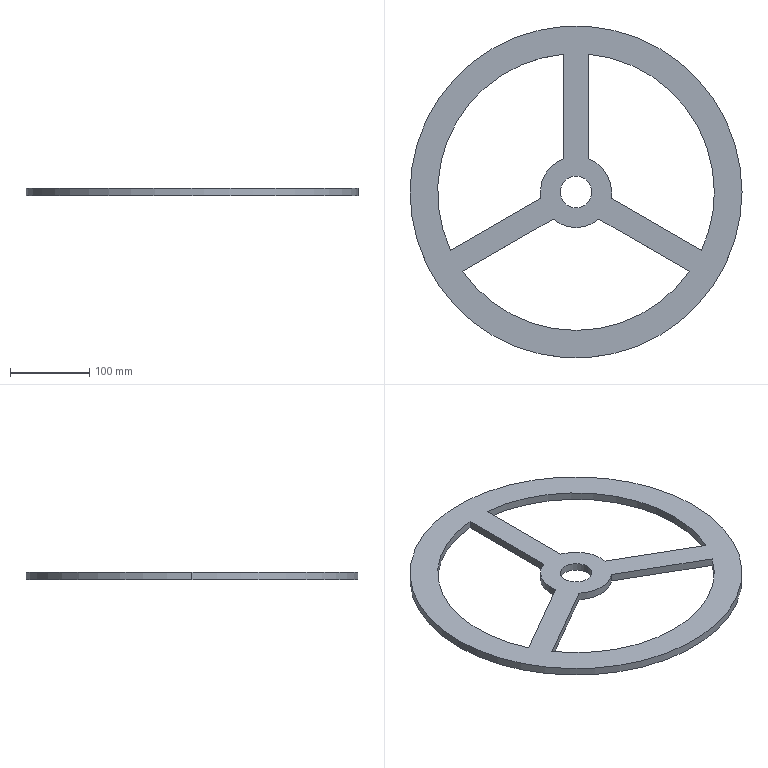Part | SolidWorks | features BaseBody 1 | 1 solid | 20 faces | box 420 x 420 x 10 mm | volume 593937 mm3 | cylinder 12 | plane 8 | commonest cylinder face diameters 90 x4 350 x4 40 x2 420 x2
STEP:
#1=CARTESIAN_POINT('',(20.,0.,0.));
#2=VERTEX_POINT('',#1);
#3=CARTESIAN_POINT('',(-20.,0.,0.));
#4=VERTEX_POINT('',#3);
#5=CARTESIAN_POINT('',(0.,0.,0.));
#6=DIRECTION('',(0.,0.,-1.));
#7=DIRECTION('',(1.,0.,0.));
#8=AXIS2_PLACEMENT_3D('',#5,#6,#7);
#9=CIRCLE('',#8,20.);
#10=EDGE_CURVE('',#2,#4,#9,.T.);
#11=ORIENTED_EDGE('',*,*,#10,.T.);
#12=CARTESIAN_POINT('',(-20.,0.,10.));
#13=VERTEX_POINT('',#12);
#14=CARTESIAN_POINT('',(-20.,0.,0.));
#15=DIRECTION('',(0.,0.,1.));
#16=VECTOR('',#15,1000.);
#17=LINE('',#14,#16);
#18=EDGE_CURVE('',#4,#13,#17,.T.);
#19=ORIENTED_EDGE('',*,*,#18,.T.);
#20=CARTESIAN_POINT('',(20.,0.,10.));
#21=VERTEX_POINT('',#20);
#22=CARTESIAN_POINT('',(0.,0.,10.));
#23=DIRECTION('',(0.,0.,-1.));
#24=DIRECTION('',(1.,0.,0.));
#25=AXIS2_PLACEMENT_3D('',#22,#23,#24);
#26=CIRCLE('',#25,20.);
#27=EDGE_CURVE('',#21,#13,#26,.T.);
#28=ORIENTED_EDGE('',*,*,#27,.F.);
#29=CARTESIAN_POINT('',(20.,0.,0.));
#30=DIRECTION('',(0.,0.,1.));
#31=VECTOR('',#30,1000.);
#32=LINE('',#29,#31);
#33=EDGE_CURVE('',#2,#21,#32,.T.);
#34=ORIENTED_EDGE('',*,*,#33,.F.);
#35=EDGE_LOOP('',(#11,#19,#28,#34));
#36=FACE_OUTER_BOUND('',#35,.T.);
#37=CARTESIAN_POINT('',(0.,0.,0.));
#38=DIRECTION('',(0.,0.,1.));
#39=DIRECTION('',(1.,0.,0.));
#40=AXIS2_PLACEMENT_3D('',#37,#38,#39);
#41=CYLINDRICAL_SURFACE('',#40,20.);
#42=ADVANCED_FACE('',(#36),#41,.F.);
#43=CARTESIAN_POINT('',(15.251,174.334,0.));
#44=VERTEX_POINT('',#43);
#45=CARTESIAN_POINT('',(175.,0.,0.));
#46=VERTEX_POINT('',#45);
#47=CARTESIAN_POINT('',(0.,0.,0.));
#48=DIRECTION('',(0.,0.,-1.));
#49=DIRECTION('',(1.,0.,0.));
#50=AXIS2_PLACEMENT_3D('',#47,#48,#49);
#51=CIRCLE('',#50,175.);
#52=EDGE_CURVE('',#44,#46,#51,.T.);
#53=ORIENTED_EDGE('',*,*,#52,.T.);
#54=CARTESIAN_POINT('',(175.,0.,10.));
#55=VERTEX_POINT('',#54);
#56=CARTESIAN_POINT('',(175.,0.,0.));
#57=DIRECTION('',(0.,0.,1.));
#58=VECTOR('',#57,1000.);
#59=LINE('',#56,#58);
#60=EDGE_CURVE('',#46,#55,#59,.T.);
#61=ORIENTED_EDGE('',*,*,#60,.T.);
#62=CARTESIAN_POINT('',(15.251,174.334,10.));
#63=VERTEX_POINT('',#62);
#64=CARTESIAN_POINT('',(0.,0.,10.));
#65=DIRECTION('',(0.,0.,-1.));
#66=DIRECTION('',(1.,0.,0.));
#67=AXIS2_PLACEMENT_3D('',#64,#65,#66);
#68=CIRCLE('',#67,175.);
#69=EDGE_CURVE('',#63,#55,#68,.T.);
#70=ORIENTED_EDGE('',*,*,#69,.F.);
#71=CARTESIAN_POINT('',(15.251,174.334,0.));
#72=DIRECTION('',(0.,0.,1.));
#73=VECTOR('',#72,1000.);
#74=LINE('',#71,#73);
#75=EDGE_CURVE('',#44,#63,#74,.T.);
#76=ORIENTED_EDGE('',*,*,#75,.F.);
#77=EDGE_LOOP('',(#53,#61,#70,#76));
#78=FACE_OUTER_BOUND('',#77,.T.);
#79=CARTESIAN_POINT('',(0.,0.,0.));
#80=DIRECTION('',(0.,0.,1.));
#81=DIRECTION('',(1.,0.,0.));
#82=AXIS2_PLACEMENT_3D('',#79,#80,#81);
#83=CYLINDRICAL_SURFACE('',#82,175.);
#84=ADVANCED_FACE('',(#78),#83,.F.);
#85=CARTESIAN_POINT('',(44.29,-7.961,0.));
#86=VERTEX_POINT('',#85);
#87=CARTESIAN_POINT('',(45.,0.,0.));
#88=VERTEX_POINT('',#87);
#89=CARTESIAN_POINT('',(0.,0.,0.));
#90=DIRECTION('',(0.,0.,1.));
#91=DIRECTION('',(1.,0.,0.));
#92=AXIS2_PLACEMENT_3D('',#89,#90,#91);
#93=CIRCLE('',#92,45.);
#94=EDGE_CURVE('',#86,#88,#93,.T.);
#95=ORIENTED_EDGE('',*,*,#94,.T.);
#96=CARTESIAN_POINT('',(45.,0.,10.));
#97=VERTEX_POINT('',#96);
#98=CARTESIAN_POINT('',(45.,0.,0.));
#99=DIRECTION('',(0.,0.,1.));
#100=VECTOR('',#99,1000.);
#101=LINE('',#98,#100);
#102=EDGE_CURVE('',#88,#97,#101,.T.);
#103=ORIENTED_EDGE('',*,*,#102,.T.);
#104=CARTESIAN_POINT('',(44.29,-7.961,10.));
#105=VERTEX_POINT('',#104);
#106=CARTESIAN_POINT('',(0.,0.,10.));
#107=DIRECTION('',(0.,0.,-1.));
#108=DIRECTION('',(1.,0.,0.));
#109=AXIS2_PLACEMENT_3D('',#106,#107,#108);
#110=CIRCLE('',#109,45.);
#111=EDGE_CURVE('',#97,#105,#110,.T.);
#112=ORIENTED_EDGE('',*,*,#111,.T.);
#113=CARTESIAN_POINT('',(44.29,-7.961,0.));
#114=DIRECTION('',(0.,0.,-1.));
#115=VECTOR('',#114,1000.);
#116=LINE('',#113,#115);
#117=EDGE_CURVE('',#105,#86,#116,.T.);
#118=ORIENTED_EDGE('',*,*,#117,.T.);
#119=EDGE_LOOP('',(#95,#103,#112,#118));
#120=FACE_OUTER_BOUND('',#119,.T.);
#121=CARTESIAN_POINT('',(0.,0.,0.));
#122=DIRECTION('',(0.,0.,1.));
#123=DIRECTION('',(1.,0.,0.));
#124=AXIS2_PLACEMENT_3D('',#121,#122,#123);
#125=CYLINDRICAL_SURFACE('',#124,45.);
#126=ADVANCED_FACE('',(#120),#125,.T.);
#127=CARTESIAN_POINT('',(210.,0.,0.));
#128=VERTEX_POINT('',#127);
#129=CARTESIAN_POINT('',(-210.,0.,0.));
#130=VERTEX_POINT('',#129);
#131=CARTESIAN_POINT('',(0.,0.,0.));
#132=DIRECTION('',(0.,0.,1.));
#133=DIRECTION('',(1.,0.,0.));
#134=AXIS2_PLACEMENT_3D('',#131,#132,#133);
#135=CIRCLE('',#134,210.);
#136=EDGE_CURVE('',#128,#130,#135,.T.);
#137=ORIENTED_EDGE('',*,*,#136,.T.);
#138=CARTESIAN_POINT('',(-210.,0.,10.));
#139=VERTEX_POINT('',#138);
#140=CARTESIAN_POINT('',(-210.,0.,0.));
#141=DIRECTION('',(0.,0.,1.));
#142=VECTOR('',#141,1000.);
#143=LINE('',#140,#142);
#144=EDGE_CURVE('',#130,#139,#143,.T.);
#145=ORIENTED_EDGE('',*,*,#144,.T.);
#146=CARTESIAN_POINT('',(210.,0.,10.));
#147=VERTEX_POINT('',#146);
#148=CARTESIAN_POINT('',(0.,0.,10.));
#149=DIRECTION('',(0.,0.,-1.));
#150=DIRECTION('',(1.,0.,0.));
#151=AXIS2_PLACEMENT_3D('',#148,#149,#150);
#152=CIRCLE('',#151,210.);
#153=EDGE_CURVE('',#139,#147,#152,.T.);
#154=ORIENTED_EDGE('',*,*,#153,.T.);
#155=CARTESIAN_POINT('',(210.,0.,0.));
#156=DIRECTION('',(0.,0.,1.));
#157=VECTOR('',#156,1000.);
#158=LINE('',#155,#157);
#159=EDGE_CURVE('',#128,#147,#158,.T.);
#160=ORIENTED_EDGE('',*,*,#159,.F.);
#161=EDGE_LOOP('',(#137,#145,#154,#160));
#162=FACE_OUTER_BOUND('',#161,.T.);
#163=CARTESIAN_POINT('',(0.,0.,0.));
#164=DIRECTION('',(0.,0.,1.));
#165=DIRECTION('',(1.,0.,0.));
#166=AXIS2_PLACEMENT_3D('',#163,#164,#165);
#167=CYLINDRICAL_SURFACE('',#166,210.);
#168=ADVANCED_FACE('',(#162),#167,.T.);
#169=ORIENTED_EDGE('',*,*,#10,.F.);
#170=CARTESIAN_POINT('',(0.,0.,0.));
#171=DIRECTION('',(0.,0.,-1.));
#172=DIRECTION('',(1.,0.,0.));
#173=AXIS2_PLACEMENT_3D('',#170,#171,#172);
#174=CIRCLE('',#173,20.);
#175=EDGE_CURVE('',#4,#2,#174,.T.);
#176=ORIENTED_EDGE('',*,*,#175,.F.);
#177=EDGE_LOOP('',(#169,#176));
#178=FACE_BOUND('',#177,.T.);
#179=CARTESIAN_POINT('',(-15.251,42.337,0.));
#180=VERTEX_POINT('',#179);
#181=CARTESIAN_POINT('',(-44.29,-7.961,0.));
#182=VERTEX_POINT('',#181);
#183=CARTESIAN_POINT('',(0.,0.,0.));
#184=DIRECTION('',(0.,0.,1.));
#185=DIRECTION('',(1.,0.,0.));
#186=AXIS2_PLACEMENT_3D('',#183,#184,#185);
#187=CIRCLE('',#186,45.);
#188=EDGE_CURVE('',#180,#182,#187,.T.);
#189=ORIENTED_EDGE('',*,*,#188,.F.);
#190=CARTESIAN_POINT('',(-15.251,174.334,0.));
#191=VERTEX_POINT('',#190);
#192=CARTESIAN_POINT('',(-15.251,0.,0.));
#193=DIRECTION('',(0.,-1.,0.));
#194=VECTOR('',#193,1000.);
#195=LINE('',#192,#194);
#196=EDGE_CURVE('',#191,#180,#195,.T.);
#197=ORIENTED_EDGE('',*,*,#196,.F.);
#198=CARTESIAN_POINT('',(-158.603,-73.959,0.));
#199=VERTEX_POINT('',#198);
#200=CARTESIAN_POINT('',(0.,0.,0.));
#201=DIRECTION('',(0.,0.,-1.));
#202=DIRECTION('',(1.,0.,0.));
#203=AXIS2_PLACEMENT_3D('',#200,#201,#202);
#204=CIRCLE('',#203,175.);
#205=EDGE_CURVE('',#199,#191,#204,.T.);
#206=ORIENTED_EDGE('',*,*,#205,.F.);
#207=CARTESIAN_POINT('',(-44.29,-7.961,0.));
#208=DIRECTION('',(-0.866,-0.5,0.));
#209=VECTOR('',#208,1000.);
#210=LINE('',#207,#209);
#211=EDGE_CURVE('',#182,#199,#210,.T.);
#212=ORIENTED_EDGE('',*,*,#211,.F.);
#213=EDGE_LOOP('',(#189,#197,#206,#212));
#214=FACE_BOUND('',#213,.T.);
#215=CARTESIAN_POINT('',(-29.039,-34.376,0.));
#216=VERTEX_POINT('',#215);
#217=CARTESIAN_POINT('',(29.039,-34.376,0.));
#218=VERTEX_POINT('',#217);
#219=CARTESIAN_POINT('',(0.,0.,0.));
#220=DIRECTION('',(0.,0.,1.));
#221=DIRECTION('',(1.,0.,0.));
#222=AXIS2_PLACEMENT_3D('',#219,#220,#221);
#223=CIRCLE('',#222,45.);
#224=EDGE_CURVE('',#216,#218,#223,.T.);
#225=ORIENTED_EDGE('',*,*,#224,.F.);
#226=CARTESIAN_POINT('',(-143.352,-100.375,0.));
#227=VERTEX_POINT('',#226);
#228=CARTESIAN_POINT('',(-143.352,-100.375,0.));
#229=DIRECTION('',(0.866,0.5,0.));
#230=VECTOR('',#229,1000.);
#231=LINE('',#228,#230);
#232=EDGE_CURVE('',#227,#216,#231,.T.);
#233=ORIENTED_EDGE('',*,*,#232,.F.);
#234=CARTESIAN_POINT('',(143.352,-100.375,0.));
#235=VERTEX_POINT('',#234);
#236=CARTESIAN_POINT('',(0.,0.,0.));
#237=DIRECTION('',(0.,0.,-1.));
#238=DIRECTION('',(1.,0.,0.));
#239=AXIS2_PLACEMENT_3D('',#236,#237,#238);
#240=CIRCLE('',#239,175.);
#241=EDGE_CURVE('',#235,#227,#240,.T.);
#242=ORIENTED_EDGE('',*,*,#241,.F.);
#243=CARTESIAN_POINT('',(29.039,-34.376,0.));
#244=DIRECTION('',(0.866,-0.5,0.));
#245=VECTOR('',#244,1000.);
#246=LINE('',#243,#245);
#247=EDGE_CURVE('',#218,#235,#246,.T.);
#248=ORIENTED_EDGE('',*,*,#247,.F.);
#249=EDGE_LOOP('',(#225,#233,#242,#248));
#250=FACE_BOUND('',#249,.T.);
#251=CARTESIAN_POINT('',(15.251,42.337,0.));
#252=VERTEX_POINT('',#251);
#253=CARTESIAN_POINT('',(15.251,0.,0.));
#254=DIRECTION('',(0.,1.,0.));
#255=VECTOR('',#254,1000.);
#256=LINE('',#253,#255);
#257=EDGE_CURVE('',#252,#44,#256,.T.);
#258=ORIENTED_EDGE('',*,*,#257,.F.);
#259=CARTESIAN_POINT('',(0.,0.,0.));
#260=DIRECTION('',(0.,0.,1.));
#261=DIRECTION('',(1.,0.,0.));
#262=AXIS2_PLACEMENT_3D('',#259,#260,#261);
#263=CIRCLE('',#262,45.);
#264=EDGE_CURVE('',#88,#252,#263,.T.);
#265=ORIENTED_EDGE('',*,*,#264,.F.);
#266=ORIENTED_EDGE('',*,*,#94,.F.);
#267=CARTESIAN_POINT('',(158.603,-73.959,0.));
#268=VERTEX_POINT('',#267);
#269=CARTESIAN_POINT('',(158.603,-73.959,0.));
#270=DIRECTION('',(-0.866,0.5,0.));
#271=VECTOR('',#270,1000.);
#272=LINE('',#269,#271);
#273=EDGE_CURVE('',#268,#86,#272,.T.);
#274=ORIENTED_EDGE('',*,*,#273,.F.);
#275=CARTESIAN_POINT('',(0.,0.,0.));
#276=DIRECTION('',(0.,0.,-1.));
#277=DIRECTION('',(1.,0.,0.));
#278=AXIS2_PLACEMENT_3D('',#275,#276,#277);
#279=CIRCLE('',#278,175.);
#280=EDGE_CURVE('',#46,#268,#279,.T.);
#281=ORIENTED_EDGE('',*,*,#280,.F.);
#282=ORIENTED_EDGE('',*,*,#52,.F.);
#283=EDGE_LOOP('',(#258,#265,#266,#274,#281,#282));
#284=FACE_BOUND('',#283,.T.);
#285=ORIENTED_EDGE('',*,*,#136,.F.);
#286=CARTESIAN_POINT('',(0.,0.,0.));
#287=DIRECTION('',(0.,0.,1.));
#288=DIRECTION('',(1.,0.,0.));
#289=AXIS2_PLACEMENT_3D('',#286,#287,#288);
#290=CIRCLE('',#289,210.);
#291=EDGE_CURVE('',#130,#128,#290,.T.);
#292=ORIENTED_EDGE('',*,*,#291,.F.);
#293=EDGE_LOOP('',(#285,#292));
#294=FACE_OUTER_BOUND('',#293,.T.);
#295=CARTESIAN_POINT('',(0.,0.,0.));
#296=DIRECTION('',(0.,0.,1.));
#297=DIRECTION('',(1.,0.,0.));
#298=AXIS2_PLACEMENT_3D('',#295,#296,#297);
#299=PLANE('',#298);
#300=ADVANCED_FACE('',(#178,#214,#250,#284,#294),#299,.F.);
#301=ORIENTED_EDGE('',*,*,#18,.F.);
#302=ORIENTED_EDGE('',*,*,#175,.T.);
#303=ORIENTED_EDGE('',*,*,#33,.T.);
#304=CARTESIAN_POINT('',(0.,0.,10.));
#305=DIRECTION('',(0.,0.,-1.));
#306=DIRECTION('',(1.,0.,0.));
#307=AXIS2_PLACEMENT_3D('',#304,#305,#306);
#308=CIRCLE('',#307,20.);
#309=EDGE_CURVE('',#13,#21,#308,.T.);
#310=ORIENTED_EDGE('',*,*,#309,.F.);
#311=EDGE_LOOP('',(#301,#302,#303,#310));
#312=FACE_OUTER_BOUND('',#311,.T.);
#313=CARTESIAN_POINT('',(0.,0.,0.));
#314=DIRECTION('',(0.,0.,1.));
#315=DIRECTION('',(1.,0.,0.));
#316=AXIS2_PLACEMENT_3D('',#313,#314,#315);
#317=CYLINDRICAL_SURFACE('',#316,20.);
#318=ADVANCED_FACE('',(#312),#317,.F.);
#319=CARTESIAN_POINT('',(-44.29,-7.961,10.));
#320=VERTEX_POINT('',#319);
#321=CARTESIAN_POINT('',(-44.29,-7.961,10.));
#322=DIRECTION('',(0.,0.,-1.));
#323=VECTOR('',#322,1000.);
#324=LINE('',#321,#323);
#325=EDGE_CURVE('',#320,#182,#324,.T.);
#326=ORIENTED_EDGE('',*,*,#325,.T.);
#327=ORIENTED_EDGE('',*,*,#211,.T.);
#328=CARTESIAN_POINT('',(-158.603,-73.959,10.));
#329=VERTEX_POINT('',#328);
#330=CARTESIAN_POINT('',(-158.603,-73.959,10.));
#331=DIRECTION('',(0.,0.,1.));
#332=VECTOR('',#331,1000.);
#333=LINE('',#330,#332);
#334=EDGE_CURVE('',#199,#329,#333,.T.);
#335=ORIENTED_EDGE('',*,*,#334,.T.);
#336=CARTESIAN_POINT('',(-172.381,-81.914,10.));
#337=DIRECTION('',(0.866,0.5,0.));
#338=VECTOR('',#337,1000.);
#339=LINE('',#336,#338);
#340=EDGE_CURVE('',#329,#320,#339,.T.);
#341=ORIENTED_EDGE('',*,*,#340,.T.);
#342=EDGE_LOOP('',(#326,#327,#335,#341));
#343=FACE_OUTER_BOUND('',#342,.T.);
#344=CARTESIAN_POINT('',(-172.381,-81.914,10.));
#345=DIRECTION('',(-0.5,0.866,0.));
#346=DIRECTION('',(-0.866,-0.5,0.));
#347=AXIS2_PLACEMENT_3D('',#344,#345,#346);
#348=PLANE('',#347);
#349=ADVANCED_FACE('',(#343),#348,.T.);
#350=CARTESIAN_POINT('',(-15.251,42.337,10.));
#351=VERTEX_POINT('',#350);
#352=CARTESIAN_POINT('',(-15.251,42.337,0.));
#353=DIRECTION('',(0.,0.,-1.));
#354=VECTOR('',#353,1000.);
#355=LINE('',#352,#354);
#356=EDGE_CURVE('',#351,#180,#355,.T.);
#357=ORIENTED_EDGE('',*,*,#356,.T.);
#358=ORIENTED_EDGE('',*,*,#188,.T.);
#359=ORIENTED_EDGE('',*,*,#325,.F.);
#360=CARTESIAN_POINT('',(0.,0.,10.));
#361=DIRECTION('',(0.,0.,-1.));
#362=DIRECTION('',(1.,0.,0.));
#363=AXIS2_PLACEMENT_3D('',#360,#361,#362);
#364=CIRCLE('',#363,45.);
#365=EDGE_CURVE('',#320,#351,#364,.T.);
#366=ORIENTED_EDGE('',*,*,#365,.T.);
#367=EDGE_LOOP('',(#357,#358,#359,#366));
#368=FACE_OUTER_BOUND('',#367,.T.);
#369=CARTESIAN_POINT('',(0.,0.,0.));
#370=DIRECTION('',(0.,0.,1.));
#371=DIRECTION('',(1.,0.,0.));
#372=AXIS2_PLACEMENT_3D('',#369,#370,#371);
#373=CYLINDRICAL_SURFACE('',#372,45.);
#374=ADVANCED_FACE('',(#368),#373,.T.);
#375=CARTESIAN_POINT('',(-15.251,174.334,10.));
#376=VERTEX_POINT('',#375);
#377=CARTESIAN_POINT('',(-15.251,174.334,10.));
#378=DIRECTION('',(0.,0.,-1.));
#379=VECTOR('',#378,1000.);
#380=LINE('',#377,#379);
#381=EDGE_CURVE('',#376,#191,#380,.T.);
#382=ORIENTED_EDGE('',*,*,#381,.T.);
#383=ORIENTED_EDGE('',*,*,#196,.T.);
#384=ORIENTED_EDGE('',*,*,#356,.F.);
#385=CARTESIAN_POINT('',(-15.251,27.735,10.));
#386=DIRECTION('',(0.,1.,0.));
#387=VECTOR('',#386,1000.);
#388=LINE('',#385,#387);
#389=EDGE_CURVE('',#351,#376,#388,.T.);
#390=ORIENTED_EDGE('',*,*,#389,.T.);
#391=EDGE_LOOP('',(#382,#383,#384,#390));
#392=FACE_OUTER_BOUND('',#391,.T.);
#393=CARTESIAN_POINT('',(-15.251,27.735,10.));
#394=DIRECTION('',(-1.,0.,0.));
#395=DIRECTION('',(0.,-1.,0.));
#396=AXIS2_PLACEMENT_3D('',#393,#394,#395);
#397=PLANE('',#396);
#398=ADVANCED_FACE('',(#392),#397,.T.);
#399=ORIENTED_EDGE('',*,*,#205,.T.);
#400=ORIENTED_EDGE('',*,*,#381,.F.);
#401=CARTESIAN_POINT('',(0.,0.,10.));
#402=DIRECTION('',(0.,0.,-1.));
#403=DIRECTION('',(1.,0.,0.));
#404=AXIS2_PLACEMENT_3D('',#401,#402,#403);
#405=CIRCLE('',#404,175.);
#406=EDGE_CURVE('',#329,#376,#405,.T.);
#407=ORIENTED_EDGE('',*,*,#406,.F.);
#408=ORIENTED_EDGE('',*,*,#334,.F.);
#409=EDGE_LOOP('',(#399,#400,#407,#408));
#410=FACE_OUTER_BOUND('',#409,.T.);
#411=CARTESIAN_POINT('',(0.,0.,0.));
#412=DIRECTION('',(0.,0.,1.));
#413=DIRECTION('',(1.,0.,0.));
#414=AXIS2_PLACEMENT_3D('',#411,#412,#413);
#415=CYLINDRICAL_SURFACE('',#414,175.);
#416=ADVANCED_FACE('',(#410),#415,.F.);
#417=CARTESIAN_POINT('',(29.039,-34.376,10.));
#418=VERTEX_POINT('',#417);
#419=CARTESIAN_POINT('',(29.039,-34.376,10.));
#420=DIRECTION('',(0.,0.,-1.));
#421=VECTOR('',#420,1000.);
#422=LINE('',#419,#421);
#423=EDGE_CURVE('',#418,#218,#422,.T.);
#424=ORIENTED_EDGE('',*,*,#423,.T.);
#425=ORIENTED_EDGE('',*,*,#247,.T.);
#426=CARTESIAN_POINT('',(143.352,-100.375,10.));
#427=VERTEX_POINT('',#426);
#428=CARTESIAN_POINT('',(143.352,-100.375,10.));
#429=DIRECTION('',(0.,0.,1.));
#430=VECTOR('',#429,1000.);
#431=LINE('',#428,#430);
#432=EDGE_CURVE('',#235,#427,#431,.T.);
#433=ORIENTED_EDGE('',*,*,#432,.T.);
#434=CARTESIAN_POINT('',(157.13,-108.329,10.));
#435=DIRECTION('',(-0.866,0.5,0.));
#436=VECTOR('',#435,1000.);
#437=LINE('',#434,#436);
#438=EDGE_CURVE('',#427,#418,#437,.T.);
#439=ORIENTED_EDGE('',*,*,#438,.T.);
#440=EDGE_LOOP('',(#424,#425,#433,#439));
#441=FACE_OUTER_BOUND('',#440,.T.);
#442=CARTESIAN_POINT('',(157.13,-108.329,10.));
#443=DIRECTION('',(-0.5,-0.866,0.));
#444=DIRECTION('',(0.866,-0.5,0.));
#445=AXIS2_PLACEMENT_3D('',#442,#443,#444);
#446=PLANE('',#445);
#447=ADVANCED_FACE('',(#441),#446,.T.);
#448=CARTESIAN_POINT('',(-29.039,-34.376,10.));
#449=VERTEX_POINT('',#448);
#450=CARTESIAN_POINT('',(-29.039,-34.376,0.));
#451=DIRECTION('',(0.,0.,-1.));
#452=VECTOR('',#451,1000.);
#453=LINE('',#450,#452);
#454=EDGE_CURVE('',#449,#216,#453,.T.);
#455=ORIENTED_EDGE('',*,*,#454,.T.);
#456=ORIENTED_EDGE('',*,*,#224,.T.);
#457=ORIENTED_EDGE('',*,*,#423,.F.);
#458=CARTESIAN_POINT('',(0.,0.,10.));
#459=DIRECTION('',(0.,0.,-1.));
#460=DIRECTION('',(1.,0.,0.));
#461=AXIS2_PLACEMENT_3D('',#458,#459,#460);
#462=CIRCLE('',#461,45.);
#463=EDGE_CURVE('',#418,#449,#462,.T.);
#464=ORIENTED_EDGE('',*,*,#463,.T.);
#465=EDGE_LOOP('',(#455,#456,#457,#464));
#466=FACE_OUTER_BOUND('',#465,.T.);
#467=CARTESIAN_POINT('',(0.,0.,0.));
#468=DIRECTION('',(0.,0.,1.));
#469=DIRECTION('',(1.,0.,0.));
#470=AXIS2_PLACEMENT_3D('',#467,#468,#469);
#471=CYLINDRICAL_SURFACE('',#470,45.);
#472=ADVANCED_FACE('',(#466),#471,.T.);
#473=ORIENTED_EDGE('',*,*,#454,.F.);
#474=CARTESIAN_POINT('',(-143.352,-100.375,10.));
#475=VERTEX_POINT('',#474);
#476=CARTESIAN_POINT('',(-16.394,-27.075,10.));
#477=DIRECTION('',(-0.866,-0.5,0.));
#478=VECTOR('',#477,1000.);
#479=LINE('',#476,#478);
#480=EDGE_CURVE('',#449,#475,#479,.T.);
#481=ORIENTED_EDGE('',*,*,#480,.T.);
#482=CARTESIAN_POINT('',(-143.352,-100.375,10.));
#483=DIRECTION('',(0.,0.,-1.));
#484=VECTOR('',#483,1000.);
#485=LINE('',#482,#484);
#486=EDGE_CURVE('',#475,#227,#485,.T.);
#487=ORIENTED_EDGE('',*,*,#486,.T.);
#488=ORIENTED_EDGE('',*,*,#232,.T.);
#489=EDGE_LOOP('',(#473,#481,#487,#488));
#490=FACE_OUTER_BOUND('',#489,.T.);
#491=CARTESIAN_POINT('',(-16.394,-27.075,10.));
#492=DIRECTION('',(0.5,-0.866,0.));
#493=DIRECTION('',(0.866,0.5,0.));
#494=AXIS2_PLACEMENT_3D('',#491,#492,#493);
#495=PLANE('',#494);
#496=ADVANCED_FACE('',(#490),#495,.T.);
#497=ORIENTED_EDGE('',*,*,#241,.T.);
#498=ORIENTED_EDGE('',*,*,#486,.F.);
#499=CARTESIAN_POINT('',(0.,0.,10.));
#500=DIRECTION('',(0.,0.,-1.));
#501=DIRECTION('',(1.,0.,0.));
#502=AXIS2_PLACEMENT_3D('',#499,#500,#501);
#503=CIRCLE('',#502,175.);
#504=EDGE_CURVE('',#427,#475,#503,.T.);
#505=ORIENTED_EDGE('',*,*,#504,.F.);
#506=ORIENTED_EDGE('',*,*,#432,.F.);
#507=EDGE_LOOP('',(#497,#498,#505,#506));
#508=FACE_OUTER_BOUND('',#507,.T.);
#509=CARTESIAN_POINT('',(0.,0.,0.));
#510=DIRECTION('',(0.,0.,1.));
#511=DIRECTION('',(1.,0.,0.));
#512=AXIS2_PLACEMENT_3D('',#509,#510,#511);
#513=CYLINDRICAL_SURFACE('',#512,175.);
#514=ADVANCED_FACE('',(#508),#513,.F.);
#515=ORIENTED_EDGE('',*,*,#60,.F.);
#516=ORIENTED_EDGE('',*,*,#280,.T.);
#517=CARTESIAN_POINT('',(158.603,-73.959,10.));
#518=VERTEX_POINT('',#517);
#519=CARTESIAN_POINT('',(158.603,-73.959,0.));
#520=DIRECTION('',(0.,0.,-1.));
#521=VECTOR('',#520,1000.);
#522=LINE('',#519,#521);
#523=EDGE_CURVE('',#518,#268,#522,.T.);
#524=ORIENTED_EDGE('',*,*,#523,.F.);
#525=CARTESIAN_POINT('',(0.,0.,10.));
#526=DIRECTION('',(0.,0.,-1.));
#527=DIRECTION('',(1.,0.,0.));
#528=AXIS2_PLACEMENT_3D('',#525,#526,#527);
#529=CIRCLE('',#528,175.);
#530=EDGE_CURVE('',#55,#518,#529,.T.);
#531=ORIENTED_EDGE('',*,*,#530,.F.);
#532=EDGE_LOOP('',(#515,#516,#524,#531));
#533=FACE_OUTER_BOUND('',#532,.T.);
#534=CARTESIAN_POINT('',(0.,0.,0.));
#535=DIRECTION('',(0.,0.,1.));
#536=DIRECTION('',(1.,0.,0.));
#537=AXIS2_PLACEMENT_3D('',#534,#535,#536);
#538=CYLINDRICAL_SURFACE('',#537,175.);
#539=ADVANCED_FACE('',(#533),#538,.F.);
#540=ORIENTED_EDGE('',*,*,#75,.T.);
#541=CARTESIAN_POINT('',(15.251,42.337,10.));
#542=VERTEX_POINT('',#541);
#543=CARTESIAN_POINT('',(15.251,190.243,10.));
#544=DIRECTION('',(0.,-1.,0.));
#545=VECTOR('',#544,1000.);
#546=LINE('',#543,#545);
#547=EDGE_CURVE('',#63,#542,#546,.T.);
#548=ORIENTED_EDGE('',*,*,#547,.T.);
#549=CARTESIAN_POINT('',(15.251,42.337,10.));
#550=DIRECTION('',(0.,0.,-1.));
#551=VECTOR('',#550,1000.);
#552=LINE('',#549,#551);
#553=EDGE_CURVE('',#542,#252,#552,.T.);
#554=ORIENTED_EDGE('',*,*,#553,.T.);
#555=ORIENTED_EDGE('',*,*,#257,.T.);
#556=EDGE_LOOP('',(#540,#548,#554,#555));
#557=FACE_OUTER_BOUND('',#556,.T.);
#558=CARTESIAN_POINT('',(15.251,190.243,10.));
#559=DIRECTION('',(1.,0.,0.));
#560=DIRECTION('',(0.,1.,0.));
#561=AXIS2_PLACEMENT_3D('',#558,#559,#560);
#562=PLANE('',#561);
#563=ADVANCED_FACE('',(#557),#562,.T.);
#564=ORIENTED_EDGE('',*,*,#102,.F.);
#565=ORIENTED_EDGE('',*,*,#264,.T.);
#566=ORIENTED_EDGE('',*,*,#553,.F.);
#567=CARTESIAN_POINT('',(0.,0.,10.));
#568=DIRECTION('',(0.,0.,-1.));
#569=DIRECTION('',(1.,0.,0.));
#570=AXIS2_PLACEMENT_3D('',#567,#568,#569);
#571=CIRCLE('',#570,45.);
#572=EDGE_CURVE('',#542,#97,#571,.T.);
#573=ORIENTED_EDGE('',*,*,#572,.T.);
#574=EDGE_LOOP('',(#564,#565,#566,#573));
#575=FACE_OUTER_BOUND('',#574,.T.);
#576=CARTESIAN_POINT('',(0.,0.,0.));
#577=DIRECTION('',(0.,0.,1.));
#578=DIRECTION('',(1.,0.,0.));
#579=AXIS2_PLACEMENT_3D('',#576,#577,#578);
#580=CYLINDRICAL_SURFACE('',#579,45.);
#581=ADVANCED_FACE('',(#575),#580,.T.);
#582=ORIENTED_EDGE('',*,*,#117,.F.);
#583=CARTESIAN_POINT('',(31.645,-0.6599,10.));
#584=DIRECTION('',(0.866,-0.5,0.));
#585=VECTOR('',#584,1000.);
#586=LINE('',#583,#585);
#587=EDGE_CURVE('',#105,#518,#586,.T.);
#588=ORIENTED_EDGE('',*,*,#587,.T.);
#589=ORIENTED_EDGE('',*,*,#523,.T.);
#590=ORIENTED_EDGE('',*,*,#273,.T.);
#591=EDGE_LOOP('',(#582,#588,#589,#590));
#592=FACE_OUTER_BOUND('',#591,.T.);
#593=CARTESIAN_POINT('',(31.645,-0.6599,10.));
#594=DIRECTION('',(0.5,0.866,0.));
#595=DIRECTION('',(-0.866,0.5,0.));
#596=AXIS2_PLACEMENT_3D('',#593,#594,#595);
#597=PLANE('',#596);
#598=ADVANCED_FACE('',(#592),#597,.T.);
#599=ORIENTED_EDGE('',*,*,#144,.F.);
#600=ORIENTED_EDGE('',*,*,#291,.T.);
#601=ORIENTED_EDGE('',*,*,#159,.T.);
#602=CARTESIAN_POINT('',(0.,0.,10.));
#603=DIRECTION('',(0.,0.,-1.));
#604=DIRECTION('',(1.,0.,0.));
#605=AXIS2_PLACEMENT_3D('',#602,#603,#604);
#606=CIRCLE('',#605,210.);
#607=EDGE_CURVE('',#147,#139,#606,.T.);
#608=ORIENTED_EDGE('',*,*,#607,.T.);
#609=EDGE_LOOP('',(#599,#600,#601,#608));
#610=FACE_OUTER_BOUND('',#609,.T.);
#611=CARTESIAN_POINT('',(0.,0.,0.));
#612=DIRECTION('',(0.,0.,1.));
#613=DIRECTION('',(1.,0.,0.));
#614=AXIS2_PLACEMENT_3D('',#611,#612,#613);
#615=CYLINDRICAL_SURFACE('',#614,210.);
#616=ADVANCED_FACE('',(#610),#615,.T.);
#617=ORIENTED_EDGE('',*,*,#27,.T.);
#618=ORIENTED_EDGE('',*,*,#309,.T.);
#619=EDGE_LOOP('',(#617,#618));
#620=FACE_BOUND('',#619,.T.);
#621=ORIENTED_EDGE('',*,*,#547,.F.);
#622=ORIENTED_EDGE('',*,*,#69,.T.);
#623=ORIENTED_EDGE('',*,*,#530,.T.);
#624=ORIENTED_EDGE('',*,*,#587,.F.);
#625=ORIENTED_EDGE('',*,*,#111,.F.);
#626=ORIENTED_EDGE('',*,*,#572,.F.);
#627=EDGE_LOOP('',(#621,#622,#623,#624,#625,#626));
#628=FACE_BOUND('',#627,.T.);
#629=ORIENTED_EDGE('',*,*,#365,.F.);
#630=ORIENTED_EDGE('',*,*,#340,.F.);
#631=ORIENTED_EDGE('',*,*,#406,.T.);
#632=ORIENTED_EDGE('',*,*,#389,.F.);
#633=EDGE_LOOP('',(#629,#630,#631,#632));
#634=FACE_BOUND('',#633,.T.);
#635=ORIENTED_EDGE('',*,*,#463,.F.);
#636=ORIENTED_EDGE('',*,*,#438,.F.);
#637=ORIENTED_EDGE('',*,*,#504,.T.);
#638=ORIENTED_EDGE('',*,*,#480,.F.);
#639=EDGE_LOOP('',(#635,#636,#637,#638));
#640=FACE_BOUND('',#639,.T.);
#641=ORIENTED_EDGE('',*,*,#607,.F.);
#642=ORIENTED_EDGE('',*,*,#153,.F.);
#643=EDGE_LOOP('',(#641,#642));
#644=FACE_OUTER_BOUND('',#643,.T.);
#645=CARTESIAN_POINT('',(0.,0.,10.));
#646=DIRECTION('',(0.,0.,1.));
#647=DIRECTION('',(1.,0.,0.));
#648=AXIS2_PLACEMENT_3D('',#645,#646,#647);
#649=PLANE('',#648);
#650=ADVANCED_FACE('',(#620,#628,#634,#640,#644),#649,.T.);
#651=CLOSED_SHELL('',(#42,#84,#126,#168,#300,#318,#349,#374,#398,#416,#447,#472,#496,#514,#539,#563,#581,#598,#616,#650));
#652=MANIFOLD_SOLID_BREP('',#651);
#653=CARTESIAN_POINT('',(0.,0.,0.));
#654=DIRECTION('',(0.,0.,1.));
#655=DIRECTION('',(1.,0.,0.));
#656=AXIS2_PLACEMENT_3D('',#653,#654,#655);
#657=(LENGTH_UNIT()NAMED_UNIT(*)SI_UNIT(.MILLI.,.METRE.));
#658=UNCERTAINTY_MEASURE_WITH_UNIT(LENGTH_MEASURE(0.00001),#657,'','');
#659=(NAMED_UNIT(*)PLANE_ANGLE_UNIT()SI_UNIT($,.RADIAN.));
#660=(NAMED_UNIT(*)SI_UNIT($,.STERADIAN.)SOLID_ANGLE_UNIT());
#661=(GEOMETRIC_REPRESENTATION_CONTEXT(3)GLOBAL_UNCERTAINTY_ASSIGNED_CONTEXT((#658))GLOBAL_UNIT_ASSIGNED_CONTEXT((#657,#659,#660))REPRESENTATION_CONTEXT('',''));
#662=ADVANCED_BREP_SHAPE_REPRESENTATION('',(#652,#656),#661);